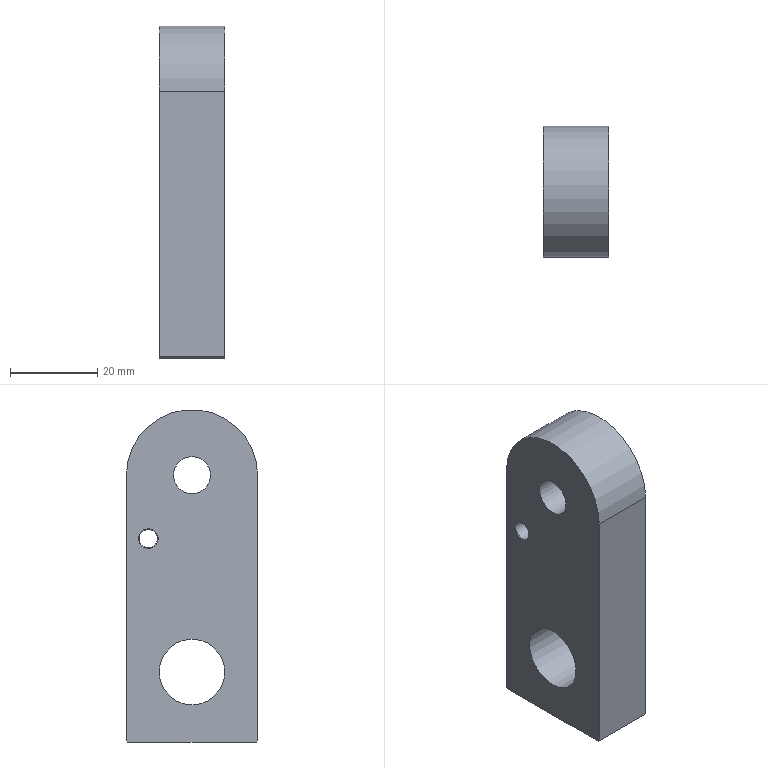NC program | NX | posted with a generic post | part box 15 x 30 x 76 mm
Lines 805 to 1774 of 31310:
(CURVE_DRIVE , TOOL : D6R0.5)
N1584 T06 M6
N1586 G53
N1588 G17 G0 G90 X-19.918 Y-1.203 S4000 M3
N1590 G43 Z50. H6
N1592 Z2.994
N1594 G94 G1 Z0.947 F1500.
N1596 Y-1.202 Z0.895
N1598 Y-1.198 Z0.843
N1600 Y-1.192 Z0.791
N1602 Y-1.184 Z0.739
N1604 X-19.919 Y-1.174 Z0.688
N1606 Y-1.161 Z0.637
N1608 Y-1.146 Z0.587
N1610 Y-1.13 Z0.537
N1612 Y-1.11 Z0.488
N1614 X-19.92 Y-1.089 Z0.44
N1616 Y-1.066 Z0.394
N1618 Y-1.041 Z0.348
N1620 X-19.921 Y-1.013 Z0.303
N1622 Y-0.984 Z0.26
N1624 Y-0.953 Z0.217
N1626 X-19.922 Y-0.92 Z0.177
N1628 Y-0.886 Z0.137
N1630 X-19.923 Y-0.849 Z0.1
N1632 Y-0.811 Z0.064
N1634 X-19.924 Y-0.772 Z0.029
N1636 Y-0.731 Z-0.004
N1638 X-19.925 Y-0.689 Z-0.034
N1640 Y-0.645 Z-0.063
N1642 X-19.926 Y-0.6 Z-0.09
N1644 Y-0.554 Z-0.116
N1646 X-19.927 Y-0.507 Z-0.139
N1648 Y-0.459 Z-0.16
N1650 X-19.928 Y-0.411 Z-0.178
N1652 X-19.929 Y-0.361 Z-0.195
N1654 Y-0.311 Z-0.21
N1656 X-19.93 Y-0.26 Z-0.222
N1658 Y-0.208 Z-0.232
N1660 X-19.931 Y-0.157 Z-0.24
N1662 X-19.932 Y-0.105 Z-0.245
N1664 Y-0.052 Z-0.249
N1666 X-19.933 Y0. Z-0.25
N1668 X-19.934 Y0.075
N1670 X-19.937 Y0.15 Z-0.249
N1672 X-19.941 Y0.226 Z-0.25
N1674 X-19.948 Y0.301
N1676 X-19.956 Y0.375
N1678 X-19.966 Y0.45 Z-0.249
N1680 X-19.972 Y0.487 Z-0.25
N1682 X-19.978 Y0.524 Z-0.249
N1684 X-19.992 Y0.598 Z-0.25
N1686 X-20.008 Y0.672
N1688 X-20.025 Y0.745
N1690 X-20.044 Y0.818 Z-0.249
N1692 X-20.065 Y0.89 Z-0.25
N1694 X-20.088 Y0.962
N1696 X-20.112 Y1.033
N1698 X-20.139 Y1.104 Z-0.249
N1700 X-20.166 Y1.174 Z-0.25
N1702 X-20.196 Y1.243
N1704 X-20.227 Y1.311
N1706 X-20.26 Y1.379
N1708 X-20.278 Y1.412
N1710 X-20.295 Y1.446 Z-0.249
N1712 X-20.331 Y1.512 Z-0.25
N1714 X-20.369 Y1.577
N1716 X-20.409 Y1.641
N1718 X-20.45 Y1.704 Z-0.249
N1720 X-20.492 Y1.766 Z-0.25
N1722 X-20.537 Y1.827
N1724 X-20.582 Y1.887
N1726 X-20.629 Y1.946 Z-0.249
N1728 X-20.678 Y2.003 Z-0.25
N1730 X-20.728 Y2.06
N1732 X-20.779 Y2.115
N1734 X-20.831 Y2.169
N1736 X-20.858 Y2.195
N1738 X-20.885 Y2.221 Z-0.249
N1740 X-20.94 Y2.272 Z-0.25
N1742 X-20.997 Y2.322
N1744 X-21.054 Y2.371
N1746 X-21.113 Y2.418 Z-0.249
N1748 X-21.173 Y2.463 Z-0.25
N1750 X-21.234 Y2.508
N1752 X-21.296 Y2.55
N1754 X-21.359 Y2.591 Z-0.249
N1756 X-21.423 Y2.631 Z-0.25
N1758 X-21.488 Y2.669
N1760 X-21.554 Y2.705
N1762 X-21.621 Y2.74
N1764 X-21.655 Y2.756
N1766 X-21.689 Y2.773 Z-0.249
N1768 X-21.757 Y2.804 Z-0.25
N1770 X-21.826 Y2.834
N1772 X-21.896 Y2.861
N1774 X-21.967 Y2.888 Z-0.249
N1776 X-22.038 Y2.912 Z-0.25
N1778 X-22.11 Y2.935
N1780 X-22.182 Y2.956
N1782 X-22.255 Y2.975 Z-0.249
N1784 X-22.328 Y2.992 Z-0.25
N1786 X-22.402 Y3.008
N1788 X-22.476 Y3.022
N1790 X-22.55 Y3.034
N1792 X-22.587 Y3.039
N1794 X-22.625 Y3.044 Z-0.249
N1796 X-22.699 Y3.052 Z-0.25
N1798 X-22.774 Y3.059
N1800 X-22.85 Y3.063
N1802 X-22.925 Y3.066 Z-0.249
N1804 X-23. Y3.067 Z-0.25
N1806 X-23.075 Y3.066
N1808 X-23.15 Y3.063
N1810 X-23.226 Y3.059 Z-0.249
N1812 X-23.301 Y3.052 Z-0.25
N1814 X-23.375 Y3.044
N1816 X-23.45 Y3.034
N1818 X-23.524 Y3.022
N1820 X-23.561 Y3.015
N1822 X-23.598 Y3.008 Z-0.249
N1824 X-23.672 Y2.992 Z-0.25
N1826 X-23.745 Y2.975
N1828 X-23.818 Y2.956
N1830 X-23.89 Y2.935 Z-0.249
N1832 X-23.962 Y2.912 Z-0.25
N1834 X-24.033 Y2.888
N1836 X-24.104 Y2.861
N1838 X-24.174 Y2.834 Z-0.249
N1840 X-24.208 Y2.819 Z-0.25
N1842 X-24.243 Y2.804
N1844 X-24.311 Y2.773
N1846 X-24.379 Y2.74
N1848 X-24.446 Y2.705
N1850 X-24.479 Y2.687
N1852 X-24.512 Y2.669 Z-0.249
N1854 X-24.577 Y2.631 Z-0.25
N1856 X-24.641 Y2.591
N1858 X-24.704 Y2.55
N1860 X-24.766 Y2.508 Z-0.249
N1862 X-24.827 Y2.463 Z-0.25
N1864 X-24.887 Y2.418
N1866 X-24.946 Y2.371
N1868 X-25.003 Y2.322 Z-0.249
N1870 X-25.032 Y2.298 Z-0.25
N1872 X-25.06 Y2.272
N1874 X-25.115 Y2.221
N1876 X-25.169 Y2.169
N1878 X-25.221 Y2.115
N1880 X-25.247 Y2.087
N1882 X-25.272 Y2.06 Z-0.249
N1884 X-25.322 Y2.003 Z-0.25
N1886 X-25.371 Y1.946
N1888 X-25.418 Y1.887
N1890 X-25.463 Y1.827 Z-0.249
N1892 X-25.508 Y1.766 Z-0.25
N1894 X-25.55 Y1.704
N1896 X-25.591 Y1.641
N1898 X-25.631 Y1.577 Z-0.249
N1900 X-25.65 Y1.544 Z-0.25
N1902 X-25.669 Y1.512
N1904 X-25.705 Y1.446
N1906 X-25.74 Y1.379
N1908 X-25.773 Y1.311
N1910 X-25.788 Y1.277
N1912 X-25.804 Y1.243 Z-0.249
N1914 X-25.834 Y1.174 Z-0.25
N1916 X-25.861 Y1.104
N1918 X-25.888 Y1.033
N1920 X-25.912 Y0.962 Z-0.249
N1922 X-25.935 Y0.89 Z-0.25
N1924 X-25.956 Y0.818
N1926 X-25.975 Y0.745
N1928 X-25.992 Y0.672 Z-0.249
N1930 X-26. Y0.635 Z-0.25
N1932 X-26.008 Y0.598
N1934 X-26.022 Y0.524
N1936 X-26.034 Y0.45
N1938 X-26.044 Y0.375
N1940 X-26.048 Y0.338
N1942 X-26.052 Y0.301 Z-0.249
N1944 X-26.059 Y0.226 Z-0.25
N1946 X-26.063 Y0.15
N1948 X-26.066 Y0.075
N1950 X-26.067 Y0. Z-0.249
N1952 X-26.066 Y-0.075 Z-0.25
N1954 X-26.063 Y-0.15
N1956 X-26.059 Y-0.226
N1958 X-26.052 Y-0.301 Z-0.249
N1960 X-26.048 Y-0.338 Z-0.25
N1962 X-26.044 Y-0.375
N1964 X-26.034 Y-0.45
N1966 X-26.022 Y-0.524
N1968 X-26.008 Y-0.598
N1970 X-26. Y-0.635
N1972 X-25.992 Y-0.672 Z-0.249
N1974 X-25.975 Y-0.745 Z-0.25
N1976 X-25.956 Y-0.818
N1978 X-25.935 Y-0.89
N1980 X-25.912 Y-0.962 Z-0.249
N1982 X-25.888 Y-1.033 Z-0.25
N1984 X-25.861 Y-1.104
N1986 X-25.834 Y-1.174
N1988 X-25.804 Y-1.243 Z-0.249
N1990 X-25.788 Y-1.277 Z-0.25
N1992 X-25.773 Y-1.311
N1994 X-25.74 Y-1.379
N1996 X-25.705 Y-1.446
N1998 X-25.669 Y-1.512
N2000 X-25.65 Y-1.544
N2002 X-25.631 Y-1.577 Z-0.249
N2004 X-25.591 Y-1.641 Z-0.25
N2006 X-25.55 Y-1.704
N2008 X-25.508 Y-1.766
N2010 X-25.463 Y-1.827 Z-0.249
N2012 X-25.418 Y-1.887 Z-0.25
N2014 X-25.371 Y-1.946
N2016 X-25.322 Y-2.003
N2018 X-25.272 Y-2.06 Z-0.249
N2020 X-25.247 Y-2.087 Z-0.25
N2022 X-25.221 Y-2.115
N2024 X-25.169 Y-2.169
N2026 X-25.115 Y-2.221
N2028 X-25.06 Y-2.272
N2030 X-25.032 Y-2.298
N2032 X-25.003 Y-2.322 Z-0.249
N2034 X-24.946 Y-2.371 Z-0.25
N2036 X-24.887 Y-2.418
N2038 X-24.827 Y-2.463
N2040 X-24.766 Y-2.508 Z-0.249
N2042 X-24.704 Y-2.55 Z-0.25
N2044 X-24.641 Y-2.591
N2046 X-24.577 Y-2.631
N2048 X-24.512 Y-2.669 Z-0.249
N2050 X-24.479 Y-2.687 Z-0.25
N2052 X-24.446 Y-2.705
N2054 X-24.379 Y-2.74
N2056 X-24.311 Y-2.773
N2058 X-24.243 Y-2.804
N2060 X-24.208 Y-2.819
N2062 X-24.174 Y-2.834 Z-0.249
N2064 X-24.104 Y-2.861 Z-0.25
N2066 X-24.033 Y-2.888
N2068 X-23.962 Y-2.912
N2070 X-23.89 Y-2.935 Z-0.249
N2072 X-23.818 Y-2.956 Z-0.25
N2074 X-23.745 Y-2.975
N2076 X-23.672 Y-2.992
N2078 X-23.598 Y-3.008 Z-0.249
N2080 X-23.561 Y-3.015 Z-0.25
N2082 X-23.524 Y-3.022
N2084 X-23.45 Y-3.034
N2086 X-23.375 Y-3.044
N2088 X-23.301 Y-3.052
N2090 X-23.226 Y-3.059 Z-0.249
N2092 X-23.15 Y-3.063 Z-0.25
N2094 X-23.075 Y-3.066
N2096 X-23. Y-3.067
N2098 X-22.925 Y-3.066 Z-0.249
N2100 X-22.85 Y-3.063 Z-0.25
N2102 X-22.774 Y-3.059
N2104 X-22.699 Y-3.052
N2106 X-22.625 Y-3.044 Z-0.249
N2108 X-22.587 Y-3.039 Z-0.25
N2110 X-22.55 Y-3.034
N2112 X-22.476 Y-3.022
N2114 X-22.402 Y-3.008
N2116 X-22.328 Y-2.992
N2118 X-22.255 Y-2.975 Z-0.249
N2120 X-22.182 Y-2.956 Z-0.25
N2122 X-22.11 Y-2.935
N2124 X-22.038 Y-2.912
N2126 X-21.967 Y-2.888 Z-0.249
N2128 X-21.896 Y-2.861 Z-0.25
N2130 X-21.826 Y-2.834
N2132 X-21.757 Y-2.804
N2134 X-21.689 Y-2.773 Z-0.249
N2136 X-21.655 Y-2.756 Z-0.25
N2138 X-21.621 Y-2.74
N2140 X-21.554 Y-2.705
N2142 X-21.488 Y-2.669
N2144 X-21.423 Y-2.631
N2146 X-21.359 Y-2.591 Z-0.249
N2148 X-21.296 Y-2.55 Z-0.25
N2150 X-21.234 Y-2.508
N2152 X-21.173 Y-2.463
N2154 X-21.113 Y-2.418 Z-0.249
N2156 X-21.054 Y-2.371 Z-0.25
N2158 X-20.997 Y-2.322
N2160 X-20.94 Y-2.272
N2162 X-20.885 Y-2.221 Z-0.249
N2164 X-20.858 Y-2.195 Z-0.25
N2166 X-20.831 Y-2.169
N2168 X-20.779 Y-2.115
N2170 X-20.728 Y-2.06
N2172 X-20.678 Y-2.003
N2174 X-20.629 Y-1.946 Z-0.249
N2176 X-20.582 Y-1.887 Z-0.25
N2178 X-20.537 Y-1.827
N2180 X-20.492 Y-1.766
N2182 X-20.45 Y-1.704 Z-0.249
N2184 X-20.409 Y-1.641 Z-0.25
N2186 X-20.369 Y-1.577
N2188 X-20.331 Y-1.512
N2190 X-20.295 Y-1.446 Z-0.249
N2192 X-20.278 Y-1.412 Z-0.25
N2194 X-20.26 Y-1.379
N2196 X-20.227 Y-1.311
N2198 X-20.196 Y-1.243
N2200 X-20.166 Y-1.174
N2202 X-20.139 Y-1.104 Z-0.249
N2204 X-20.112 Y-1.033 Z-0.25
N2206 X-20.088 Y-0.962
N2208 X-20.065 Y-0.89
N2210 X-20.044 Y-0.818 Z-0.249
N2212 X-20.025 Y-0.745 Z-0.25
N2214 X-20.008 Y-0.672
N2216 X-19.992 Y-0.598
N2218 X-19.978 Y-0.524 Z-0.249
N2220 X-19.972 Y-0.487 Z-0.25
N2222 X-19.966 Y-0.45 Z-0.249
N2224 X-19.956 Y-0.375 Z-0.25
N2226 X-19.948 Y-0.301
N2228 X-19.941 Y-0.226
N2230 X-19.937 Y-0.15 Z-0.249
N2232 X-19.934 Y-0.075 Z-0.25
N2234 X-19.933 Y0.
N2236 X-19.934 Y0.075
N2238 X-19.937 Y0.15
N2240 X-19.942 Y0.226 Z-0.251
N2242 X-19.949 Y0.301
N2244 X-19.957 Y0.375
N2246 X-19.962 Y0.413 Z-0.252
N2248 X-19.967 Y0.45
N2250 X-19.973 Y0.487
N2252 X-19.98 Y0.524
N2254 X-19.994 Y0.598 Z-0.253
N2256 X-20.009 Y0.672
N2258 X-20.027 Y0.745
N2260 X-20.046 Y0.817 Z-0.254
N2262 X-20.068 Y0.89
N2264 X-20.09 Y0.961 Z-0.255
N2266 X-20.103 Y0.997 Z-0.254
N2268 X-20.115 Y1.032 Z-0.255
N2270 X-20.142 Y1.103
N2272 X-20.17 Y1.172
N2274 X-20.199 Y1.241 Z-0.256
N2276 X-20.215 Y1.276
N2278 X-20.223 Y1.293
N2280 X-20.231 Y1.31
N2282 X-20.264 Y1.377 Z-0.257
N2284 X-20.281 Y1.411
N2286 X-20.299 Y1.444
N2288 X-20.335 Y1.51
N2290 X-20.373 Y1.574 Z-0.258
N2292 X-20.413 Y1.638
N2294 X-20.454 Y1.701
N2296 X-20.497 Y1.763 Z-0.259
N2298 X-20.519 Y1.793
N2300 X-20.541 Y1.824
N2302 X-20.587 Y1.883 Z-0.26
N2304 X-20.634 Y1.942
N2306 X-20.682 Y1.999
N2308 X-20.707 Y2.027
N2310 X-20.72 Y2.041 Z-0.261
N2312 X-20.732 Y2.055
N2314 X-20.784 Y2.11
N2316 X-20.836 Y2.164
N2318 X-20.863 Y2.19 Z-0.262
N2320 X-20.89 Y2.216
N2322 X-20.945 Y2.267
N2324 X-21.002 Y2.317 Z-0.263
N2326 X-21.059 Y2.365
N2328 X-21.118 Y2.412
N2330 X-21.178 Y2.457 Z-0.264
N2332 X-21.239 Y2.501
N2334 X-21.301 Y2.543
N2336 X-21.364 Y2.584 Z-0.265
N2338 X-21.396 Y2.604
N2340 X-21.428 Y2.623
N2342 X-21.493 Y2.661 Z-0.266
N2344 X-21.559 Y2.697
N2346 X-21.625 Y2.731
N2348 X-21.659 Y2.747 Z-0.267
N2350 X-21.693 Y2.764
N2352 X-21.761 Y2.795
N2354 X-21.83 Y2.824
N2356 X-21.9 Y2.852 Z-0.268
N2358 X-21.935 Y2.865
N2360 X-21.97 Y2.878
N2362 X-22.041 Y2.902
N2364 X-22.113 Y2.924 Z-0.269
N2366 X-22.185 Y2.945
N2368 X-22.258 Y2.964
N2370 X-22.331 Y2.981 Z-0.27
N2372 X-22.404 Y2.996
N2374 X-22.478 Y3.01 Z-0.271
N2376 X-22.515 Y3.016
N2378 X-22.552 Y3.022
N2380 X-22.589 Y3.027
N2382 X-22.626 Y3.031
N2384 X-22.701 Y3.039 Z-0.272
N2386 X-22.775 Y3.046
N2388 X-22.813 Y3.048
N2390 X-22.831 Y3.049 Z-0.273
N2392 X-22.85 Y3.05 Z-0.272
N2394 X-22.925 Y3.053 Z-0.273
N2396 X-23.
N2398 X-23.075 Y3.052 Z-0.274
N2400 X-23.15 Y3.049
N2402 X-23.225 Y3.044
N2404 X-23.299 Y3.038 Z-0.275
N2406 X-23.374 Y3.029
N2408 X-23.411 Y3.024
N2410 X-23.448 Y3.019 Z-0.276
N2412 X-23.522 Y3.007
N2414 X-23.559 Y3.
N2416 X-23.595 Y2.993
N2418 X-23.669 Y2.977 Z-0.277
N2420 X-23.705 Y2.969
N2422 X-23.723 Y2.964
N2424 X-23.732 Y2.962
N2426 X-23.741 Y2.96
N2428 X-23.814 Y2.94
N2430 X-23.886 Y2.919 Z-0.278
N2432 X-23.957 Y2.897
N2434 X-24.028 Y2.872 Z-0.279
N2436 X-24.098 Y2.846
N2438 X-24.167 Y2.818
N2440 X-24.202 Y2.803
N2442 X-24.236 Y2.788
N2444 X-24.27 Y2.773 Z-0.28
N2446 X-24.304 Y2.757
N2448 X-24.371 Y2.724
N2450 X-24.437 Y2.689 Z-0.281
N2452 X-24.47 Y2.671
N2454 X-24.503 Y2.653
N2456 X-24.535 Y2.634
N2458 X-24.551 Y2.624
N2460 X-24.567 Y2.615
N2462 X-24.631 Y2.575 Z-0.282
N2464 X-24.693 Y2.534
N2466 X-24.755 Y2.492
N2468 X-24.816 Y2.448 Z-0.283
N2470 X-24.875 Y2.403
N2472 X-24.933 Y2.356 Z-0.284
N2474 X-24.99 Y2.307
N2476 X-25.018 Y2.283
N2478 X-25.046 Y2.258
N2480 X-25.101 Y2.207 Z-0.285
N2482 X-25.154 Y2.154
N2484 X-25.206 Y2.101
N2486 X-25.232 Y2.073 Z-0.286
N2488 X-25.257 Y2.046
N2490 X-25.306 Y1.989
N2492 X-25.354 Y1.932 Z-0.287
N2494 X-25.401 Y1.874
N2496 X-25.424 Y1.844
N2498 X-25.446 Y1.814
N2500 X-25.49 Y1.753 Z-0.288
N2502 X-25.532 Y1.692
N2504 X-25.572 Y1.629
N2506 X-25.611 Y1.565 Z-0.289
N2508 X-25.63 Y1.533
N2510 X-25.649 Y1.5
N2512 X-25.684 Y1.435 Z-0.29
N2514 X-25.719 Y1.368
N2516 X-25.735 Y1.335
N2518 X-25.751 Y1.301
N2520 X-25.767 Y1.267 Z-0.291
N2522 X-25.782 Y1.233
N2524 X-25.811 Y1.165
N2526 X-25.839 Y1.095 Z-0.292
N2528 X-25.852 Y1.06
N2530 X-25.858 Y1.043
N2532 X-25.865 Y1.025
N2534 X-25.889 Y0.954
N2536 X-25.911 Y0.883
N2538 X-25.932 Y0.811 Z-0.293
N2540 X-25.951 Y0.739
N2542 X-25.968 Y0.666 Z-0.294
N2544 X-25.976 Y0.63
N2546 X-25.983 Y0.593
N2548 X-25.996 Y0.52
N2550 X-26.002 Y0.483
N2552 X-26.008 Y0.446 Z-0.295
N2554 X-26.018 Y0.372
N2556 X-26.022 Y0.335
N2558 X-26.026 Y0.298
N2560 X-26.032 Y0.224 Z-0.296
N2562 X-26.034 Y0.186
N2564 X-26.035 Y0.168
N2566 X-26.036 Y0.149
N2568 X-26.039 Y0.075 Z-0.297
N2570 X-26.04 Y0.
N2572 X-26.039 Y-0.075
N2574 X-26.036 Y-0.149 Z-0.298
N2576 X-26.031 Y-0.224
N2578 X-26.024 Y-0.298
N2580 X-26.02 Y-0.335 Z-0.299
N2582 X-26.016 Y-0.372
N2584 X-26.005 Y-0.446
N2586 X-25.993 Y-0.519 Z-0.3
N2588 X-25.98 Y-0.593
N2590 X-25.972 Y-0.629
N2592 X-25.964 Y-0.666
N2594 X-25.955 Y-0.702
N2596 X-25.951 Y-0.72
N2598 X-25.946 Y-0.738 Z-0.301
N2600 X-25.927 Y-0.81
N2602 X-25.906 Y-0.882
N2604 X-25.884 Y-0.953 Z-0.302
N2606 X-25.859 Y-1.023
N2608 X-25.833 Y-1.093 Z-0.303
N2610 X-25.805 Y-1.162
N2612 X-25.776 Y-1.23
N2614 X-25.76 Y-1.264 Z-0.304
N2616 X-25.744 Y-1.298
N2618 X-25.711 Y-1.365
N2620 X-25.677 Y-1.431
N2622 X-25.641 Y-1.496 Z-0.305
N2624 X-25.622 Y-1.528
N2626 X-25.603 Y-1.56
N2628 X-25.564 Y-1.624
N2630 X-25.523 Y-1.686 Z-0.306
N2632 X-25.481 Y-1.747
N2634 X-25.459 Y-1.777
N2636 X-25.437 Y-1.807
N2638 X-25.392 Y-1.867 Z-0.307
N2640 X-25.345 Y-1.925
N2642 X-25.297 Y-1.981 Z-0.308
N2644 X-25.272 Y-2.009
N2646 X-25.26 Y-2.023
N2648 X-25.247 Y-2.037
N2650 X-25.222 Y-2.064
N2652 X-25.197 Y-2.091
N2654 X-25.145 Y-2.145 Z-0.309
N2656 X-25.091 Y-2.196
N2658 X-25.064 Y-2.222
N2660 X-25.036 Y-2.247
N2662 X-25.009 Y-2.272 Z-0.31
N2664 X-24.981 Y-2.296
N2666 X-24.923 Y-2.344
N2668 X-24.865 Y-2.39 Z-0.311
N2670 X-24.836 Y-2.413
N2672 X-24.806 Y-2.435
N2674 X-24.745 Y-2.478
N2676 X-24.684 Y-2.52 Z-0.312
N2678 X-24.622 Y-2.561
N2680 X-24.59 Y-2.58
N2682 X-24.574 Y-2.59
N2684 X-24.558 Y-2.599 Z-0.313
N2686 X-24.494 Y-2.637
N2688 X-24.461 Y-2.655
N2690 X-24.428 Y-2.672
N2692 X-24.362 Y-2.706 Z-0.314
N2694 X-24.329 Y-2.723
N2696 X-24.295 Y-2.739
N2698 X-24.228 Y-2.77
N2700 X-24.159 Y-2.799 Z-0.315
N2702 X-24.09 Y-2.826
N2704 X-24.055 Y-2.839
N2706 X-24.038 Y-2.846
N2708 X-24.02 Y-2.852 Z-0.316
N2710 X-23.95 Y-2.876
N2712 X-23.879 Y-2.898
N2714 X-23.808 Y-2.919 Z-0.317
N2716 X-23.736 Y-2.937
N2718 X-23.663 Y-2.954
N2720 X-23.591 Y-2.97 Z-0.318
N2722 X-23.554 Y-2.976
N2724 X-23.518 Y-2.983
N2726 X-23.444 Y-2.994
N2728 X-23.371 Y-3.004 Z-0.319
N2730 X-23.297 Y-3.012
N2732 X-23.223 Y-3.018
N2734 X-23.186 Y-3.021 Z-0.32
N2736 X-23.148 Y-3.023
N2738 X-23.074 Y-3.025
N2740 X-23. Y-3.026 Z-0.321
N2742 X-22.926 Y-3.025
N2744 X-22.852 Y-3.022
N2746 X-22.777 Y-3.017 Z-0.322
N2748 X-22.703 Y-3.011
N2750 X-22.63 Y-3.002
N2752 X-22.593 Y-2.997 Z-0.323
N2754 X-22.556 Y-2.992
N2756 X-22.483 Y-2.98
N2758 X-22.41 Y-2.966 Z-0.324
N2760 X-22.337 Y-2.951
N2762 X-22.301 Y-2.942
N2764 X-22.265 Y-2.933
N2766 X-22.194 Y-2.914 Z-0.325
N2768 X-22.122 Y-2.893
N2770 X-22.052 Y-2.871
N2772 X-22.017 Y-2.859 Z-0.326
N2774 X-21.982 Y-2.846
N2776 X-21.912 Y-2.82
N2778 X-21.843 Y-2.792 Z-0.327
N2780 X-21.775 Y-2.763
N2782 X-21.741 Y-2.748
N2784 X-21.708 Y-2.732
N2786 X-21.674 Y-2.716 Z-0.328
N2788 X-21.641 Y-2.699
N2790 X-21.576 Y-2.665
N2792 X-21.511 Y-2.629
N2794 X-21.447 Y-2.591 Z-0.329
N2796 X-21.384 Y-2.552
N2798 X-21.322 Y-2.512 Z-0.33
N2800 X-21.261 Y-2.47
N2802 X-21.231 Y-2.448
N2804 X-21.201 Y-2.426
N2806 X-21.142 Y-2.381 Z-0.331
N2808 X-21.084 Y-2.334
N2810 X-21.028 Y-2.287
N2812 X-21. Y-2.262
N2814 X-20.986 Y-2.25 Z-0.332
N2816 X-20.972 Y-2.237
N2818 X-20.918 Y-2.187
N2820 X-20.891 Y-2.161
N2822 X-20.865 Y-2.135
N2824 X-20.814 Y-2.082 Z-0.333
N2826 X-20.763 Y-2.027
N2828 X-20.714 Y-1.972 Z-0.334
N2830 X-20.667 Y-1.915
N2832 X-20.621 Y-1.857
N2834 X-20.598 Y-1.827
N2836 X-20.576 Y-1.798 Z-0.335
N2838 X-20.533 Y-1.738
N2840 X-20.491 Y-1.676
N2842 X-20.451 Y-1.614 Z-0.336
N2844 X-20.431 Y-1.583
N2846 X-20.422 Y-1.567
N2848 X-20.412 Y-1.551
N2850 X-20.375 Y-1.487 Z-0.337
N2852 X-20.34 Y-1.422
N2854 X-20.322 Y-1.389
N2856 X-20.306 Y-1.356
N2858 X-20.273 Y-1.29 Z-0.338
N2860 X-20.243 Y-1.222
N2862 X-20.214 Y-1.154
N2864 X-20.187 Y-1.085 Z-0.339
N2866 X-20.161 Y-1.016
N2868 X-20.137 Y-0.946 Z-0.34
N2870 X-20.115 Y-0.875
N2872 X-20.095 Y-0.804
N2874 X-20.085 Y-0.768 Z-0.341
N2876 X-20.08 Y-0.75 Z-0.34
N2878 X-20.076 Y-0.732 Z-0.341
N2880 X-20.059 Y-0.66
N2882 X-20.044 Y-0.588
N2884 X-20.031 Y-0.515 Z-0.342
N2886 X-20.025 Y-0.479
N2888 X-20.019 Y-0.442
N2890 X-20.009 Y-0.369
N2892 X-20.001 Y-0.295 Z-0.343
N2894 X-19.995 Y-0.222
N2896 X-19.993 Y-0.185
N2898 X-19.991 Y-0.148
N2900 X-19.988 Y-0.074 Z-0.344
N2902 Y0.
N2904 X-19.989 Y0.074 Z-0.345
N2906 X-19.992 Y0.148
N2908 X-19.996 Y0.222
N2910 X-20.003 Y0.295 Z-0.346
N2912 X-20.011 Y0.369
N2914 X-20.016 Y0.405
N2916 X-20.022 Y0.442
N2918 X-20.027 Y0.478 Z-0.347
N2920 X-20.033 Y0.515
N2922 X-20.047 Y0.587
N2924 X-20.063 Y0.66 Z-0.348
N2926 X-20.08 Y0.731
N2928 X-20.099 Y0.803
N2930 X-20.12 Y0.874 Z-0.349
N2932 X-20.142 Y0.944
N2934 X-20.154 Y0.979
N2936 X-20.167 Y1.014
N2938 X-20.192 Y1.083 Z-0.35
N2940 X-20.22 Y1.151
N2942 X-20.249 Y1.219
N2944 X-20.265 Y1.253
N2946 X-20.272 Y1.27 Z-0.351
N2948 X-20.28 Y1.286
N2950 X-20.313 Y1.353
N2952 X-20.33 Y1.385
N2954 X-20.347 Y1.418
N2956 X-20.383 Y1.483 Z-0.352
N2958 X-20.42 Y1.546
N2960 X-20.459 Y1.609
N2962 X-20.499 Y1.671 Z-0.353
N2964 X-20.541 Y1.732
N2966 X-20.563 Y1.762
N2968 X-20.585 Y1.791 Z-0.354
N2970 X-20.63 Y1.85
N2972 X-20.676 Y1.907
N2974 X-20.724 Y1.964 Z-0.355
N2976 X-20.748 Y1.991
N2978 X-20.76 Y2.005
N2980 X-20.773 Y2.019
N2982 X-20.823 Y2.073
N2984 X-20.875 Y2.125 Z-0.356
N2986 X-20.901 Y2.151
N2988 X-20.928 Y2.177
N2990 X-20.982 Y2.227 Z-0.357
N2992 X-21.037 Y2.275
N2994 X-21.094 Y2.323
N2996 X-21.151 Y2.369
N2998 X-21.21 Y2.413 Z-0.358
N3000 X-21.27 Y2.456
N3002 X-21.331 Y2.498 Z-0.359
N3004 X-21.393 Y2.538
N3006 X-21.424 Y2.557
N3008 X-21.456 Y2.576
N3010 X-21.52 Y2.613 Z-0.36
N3012 X-21.584 Y2.649
N3014 X-21.65 Y2.682
N3016 X-21.683 Y2.699 Z-0.361
N3018 X-21.716 Y2.714
N3020 X-21.783 Y2.745
N3022 X-21.851 Y2.774 Z-0.362
N3024 X-21.92 Y2.801
N3026 X-21.954 Y2.814
N3028 X-21.989 Y2.826
N3030 X-22.058 Y2.85 Z-0.363
N3032 X-22.129 Y2.872
N3034 X-22.2 Y2.893
N3036 X-22.271 Y2.911 Z-0.364
N3038 X-22.342 Y2.928
N3040 X-22.415 Y2.943
N3042 X-22.487 Y2.956 Z-0.365
N3044 X-22.523 Y2.962
N3046 X-22.56 Y2.968
N3048 X-22.596 Y2.973
N3050 X-22.633 Y2.978
N3052 X-22.706 Y2.985 Z-0.366
N3054 X-22.779 Y2.992
N3056 X-22.816 Y2.994
N3058 X-22.834 Y2.995 Z-0.367
N3060 X-22.853 Y2.996 Z-0.366
N3062 X-22.926 Y2.998 Z-0.367
N3064 X-23. Y2.999
N3066 X-23.074 Y2.998 Z-0.368
N3068 X-23.147 Y2.995
N3070 X-23.221 Y2.99
N3072 X-23.294 Y2.984 Z-0.369
N3074 X-23.367 Y2.975
N3076 X-23.403 Y2.971
N3078 X-23.44 Y2.965
N3080 X-23.512 Y2.953 Z-0.37
N3082 X-23.549 Y2.947
N3084 X-23.585 Y2.94
N3086 X-23.657 Y2.924
N3088 X-23.693 Y2.916 Z-0.371
N3090 X-23.71 Y2.912
N3092 X-23.719 Y2.909
N3094 X-23.728 Y2.907
N3096 X-23.799 Y2.888
N3098 X-23.87 Y2.868
N3100 X-23.94 Y2.845 Z-0.372
N3102 X-24.009 Y2.821
N3104 X-24.078 Y2.795 Z-0.373
N3106 X-24.146 Y2.768
N3108 X-24.214 Y2.739
N3110 X-24.247 Y2.723
N3112 X-24.281 Y2.708 Z-0.374
N3114 X-24.347 Y2.675
N3116 X-24.412 Y2.641
N3118 X-24.444 Y2.624 Z-0.375
N3120 X-24.476 Y2.606
N3122 X-24.508 Y2.587
N3124 X-24.524 Y2.578
N3126 X-24.539 Y2.568
N3128 X-24.602 Y2.53 Z-0.376
N3130 X-24.663 Y2.489
N3132 X-24.724 Y2.448
N3134 X-24.783 Y2.405 Z-0.377
N3136 X-24.842 Y2.36
N3138 X-24.899 Y2.314
N3140 X-24.955 Y2.266 Z-0.378
N3142 X-24.983 Y2.242
N3144 X-25.01 Y2.218
N3146 X-25.064 Y2.167
N3148 X-25.116 Y2.116 Z-0.379
N3150 X-25.167 Y2.063
N3152 X-25.192 Y2.036
N3154 X-25.217 Y2.009
N3156 X-25.265 Y1.954 Z-0.38
N3158 X-25.313 Y1.898
N3160 X-25.358 Y1.84
N3162 X-25.381 Y1.811 Z-0.381
N3164 X-25.403 Y1.782
N3166 X-25.445 Y1.722
N3168 X-25.487 Y1.662 Z-0.382
N3170 X-25.527 Y1.6
N3172 X-25.565 Y1.537
N3174 X-25.584 Y1.506 Z-0.383
N3176 X-25.602 Y1.474
N3178 X-25.637 Y1.409
N3180 X-25.671 Y1.344
N3182 X-25.687 Y1.311 Z-0.384
N3184 X-25.703 Y1.278
N3186 X-25.718 Y1.245
N3188 X-25.733 Y1.211
N3190 X-25.762 Y1.144
N3192 X-25.789 Y1.076 Z-0.385
N3194 X-25.802 Y1.041
N3196 X-25.808 Y1.024
N3198 X-25.814 Y1.007
N3200 X-25.838 Y0.937
N3202 X-25.86 Y0.867 Z-0.386
N3204 X-25.88 Y0.797
N3206 X-25.898 Y0.726 Z-0.387
N3208 X-25.915 Y0.655
N3210 X-25.93 Y0.583
N3212 X-25.943 Y0.511 Z-0.388
N3214 X-25.949 Y0.475
N3216 X-25.955 Y0.438
N3218 X-25.964 Y0.366
N3220 X-25.969 Y0.329 Z-0.389
N3222 X-25.972 Y0.293
N3224 X-25.978 Y0.22
N3226 X-25.981 Y0.183
N3228 X-25.982 Y0.165
N3230 X-25.983 Y0.147 Z-0.39
N3232 X-25.985 Y0.073
N3234 X-25.986 Y0.
N3236 X-25.985 Y-0.073 Z-0.391
N3238 X-25.982 Y-0.146
N3240 X-25.977 Y-0.22
N3242 X-25.971 Y-0.293 Z-0.392
N3244 X-25.967 Y-0.329
N3246 X-25.962 Y-0.365
N3248 X-25.958 Y-0.402
N3250 X-25.952 Y-0.438
N3252 X-25.94 Y-0.51 Z-0.393
N3254 X-25.927 Y-0.582
N3256 X-25.911 Y-0.654
N3258 X-25.903 Y-0.689 Z-0.394
N3260 X-25.899 Y-0.707
N3262 X-25.894 Y-0.725
N3264 X-25.875 Y-0.796
N3266 X-25.855 Y-0.866
N3268 X-25.833 Y-0.936 Z-0.395
N3270 X-25.809 Y-1.005
N3272 X-25.783 Y-1.073 Z-0.396
N3274 X-25.755 Y-1.141
N3276 X-25.726 Y-1.209
N3278 X-25.711 Y-1.242 Z-0.397
N3280 X-25.696 Y-1.275
N3282 X-25.663 Y-1.341
N3284 X-25.63 Y-1.406
N3286 X-25.594 Y-1.47 Z-0.398
N3288 X-25.576 Y-1.501
N3290 X-25.557 Y-1.533
N3292 X-25.519 Y-1.595
N3294 X-25.478 Y-1.656 Z-0.399
N3296 X-25.437 Y-1.716
N3298 X-25.416 Y-1.746
N3300 X-25.394 Y-1.775
N3302 X-25.349 Y-1.834 Z-0.4
N3304 X-25.304 Y-1.891
N3306 X-25.256 Y-1.946 Z-0.401
N3308 X-25.232 Y-1.974
N3310 X-25.22 Y-1.987
N3312 X-25.208 Y-2.001
N3314 X-25.183 Y-2.028
N3316 X-25.158 Y-2.054
N3318 X-25.107 Y-2.107 Z-0.402
N3320 X-25.054 Y-2.158
N3322 X-25.027 Y-2.182
N3324 X-25. Y-2.207
N3326 X-24.946 Y-2.255 Z-0.403
N3328 X-24.889 Y-2.302
N3330 X-24.832 Y-2.348 Z-0.404
N3332 X-24.803 Y-2.37
N3334 X-24.774 Y-2.392
N3336 X-24.715 Y-2.435
N3338 X-24.654 Y-2.476
N3340 X-24.593 Y-2.515 Z-0.405
N3342 X-24.562 Y-2.535
N3344 X-24.546 Y-2.544
N3346 X-24.531 Y-2.554
N3348 X-24.467 Y-2.59 Z-0.406
N3350 X-24.435 Y-2.608
N3352 X-24.403 Y-2.625
N3354 X-24.338 Y-2.659
N3356 X-24.305 Y-2.675
N3358 X-24.273 Y-2.691 Z-0.407
N3360 X-24.206 Y-2.721
N3362 X-24.139 Y-2.749
N3364 X-24.071 Y-2.776 Z-0.408
N3366 X-24.037 Y-2.789
N3368 X-24.02 Y-2.795
N3370 X-24.002 Y-2.802
N3372 X-23.933 Y-2.825
N3374 X-23.864 Y-2.847 Z-0.409
N3376 X-23.793 Y-2.867
N3378 X-23.723 Y-2.885 Z-0.41
N3380 X-23.652 Y-2.902
N3382 X-23.58 Y-2.917
N3384 X-23.544 Y-2.924 Z-0.411
N3386 X-23.508 Y-2.93
N3388 X-23.436 Y-2.942
N3390 X-23.364 Y-2.951
N3392 X-23.291 Y-2.959 Z-0.412
N3394 X-23.219 Y-2.965
N3396 X-23.182 Y-2.967
N3398 X-23.146 Y-2.969
N3400 X-23.073 Y-2.972 Z-0.413
N3402 X-23. Y-2.973
N3404 X-22.927 Y-2.971
N3406 X-22.854 Y-2.969 Z-0.414
N3408 X-22.781 Y-2.964
N3410 X-22.709 Y-2.957 Z-0.415
N3412 X-22.636 Y-2.949
N3414 X-22.6 Y-2.944
N3416 X-22.564 Y-2.939
N3418 X-22.492 Y-2.927 Z-0.416
N3420 X-22.42 Y-2.914
N3422 X-22.349 Y-2.899
N3424 X-22.314 Y-2.89 Z-0.417
N3426 X-22.278 Y-2.881
N3428 X-22.208 Y-2.863
N3430 X-22.138 Y-2.842 Z-0.418
N3432 X-22.068 Y-2.82
N3434 X-22.034 Y-2.808
N3436 X-22. Y-2.796
N3438 X-21.931 Y-2.77
N3440 X-21.864 Y-2.743 Z-0.419
N3442 X-21.797 Y-2.714
N3444 X-21.764 Y-2.699
N3446 X-21.731 Y-2.684 Z-0.42
N3448 X-21.698 Y-2.668
N3450 X-21.665 Y-2.652
N3452 X-21.601 Y-2.618
N3454 X-21.537 Y-2.583 Z-0.421
N3456 X-21.474 Y-2.546
N3458 X-21.412 Y-2.507
N3460 X-21.351 Y-2.467 Z-0.422
N3462 X-21.291 Y-2.426
N3464 X-21.262 Y-2.405
N3466 X-21.232 Y-2.383
N3468 X-21.175 Y-2.339 Z-0.423
N3470 X-21.118 Y-2.293
N3472 X-21.062 Y-2.246 Z-0.424
N3474 X-21.035 Y-2.222
N3476 X-21.021 Y-2.21
N3478 X-21.008 Y-2.198
N3480 X-20.955 Y-2.148
N3482 X-20.929 Y-2.123 Z-0.425
N3484 X-20.903 Y-2.097
N3486 X-20.852 Y-2.045
N3488 X-20.803 Y-1.992
N3490 X-20.755 Y-1.937 Z-0.426
N3492 X-20.708 Y-1.881
N3494 X-20.663 Y-1.824
N3496 X-20.64 Y-1.795 Z-0.427
N3498 X-20.619 Y-1.766
N3500 X-20.576 Y-1.707
N3502 X-20.535 Y-1.647
N3504 X-20.496 Y-1.586 Z-0.428
N3506 X-20.477 Y-1.555
N3508 X-20.467 Y-1.539
N3510 X-20.458 Y-1.524
N3512 X-20.421 Y-1.461 Z-0.429
N3514 X-20.386 Y-1.397
N3516 X-20.37 Y-1.365